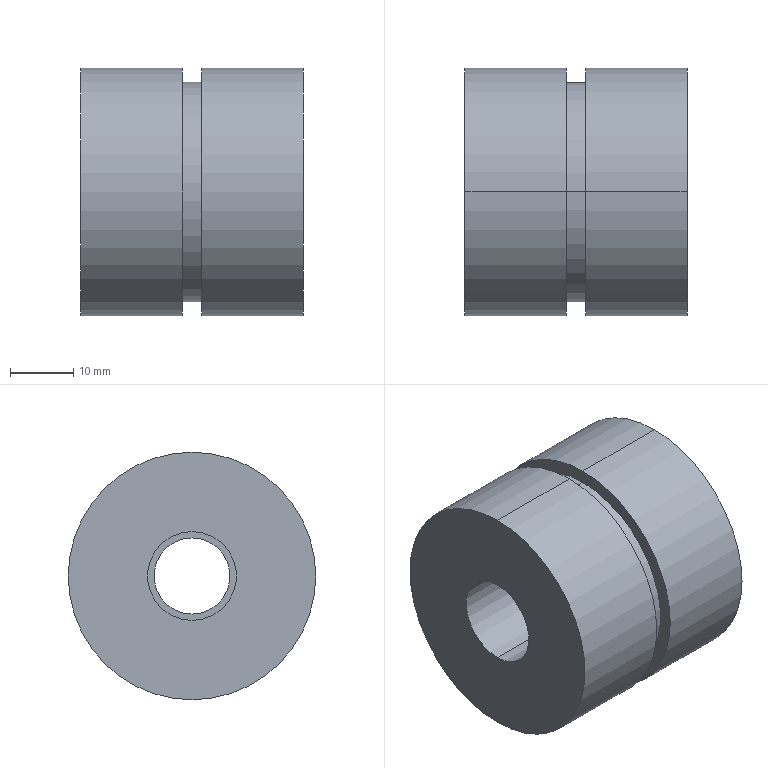Part | STEP file | PN_0042 single diaphragm coupling 39-35-14-12 | 1 solid | 15 faces | box 35 x 39 x 39 mm | volume 36443 mm3 | cylinder 10 | plane 5 | commonest cylinder face diameters 39 x4 12 x2 14 x2 34.646 x2
STEP:
#1=CARTESIAN_POINT('',(0.,0.,0.));
#2=DIRECTION('',(0.,0.,1.));
#3=DIRECTION('',(1.,0.,0.));
#4=AXIS2_PLACEMENT_3D('',#1,#2,#3);
#5=CARTESIAN_POINT('',(1.5,0.,17.323));
#6=VERTEX_POINT('',#5);
#7=CARTESIAN_POINT('',(1.5,0.,-17.323));
#8=VERTEX_POINT('',#7);
#9=CARTESIAN_POINT('',(1.5,0.,0.));
#10=DIRECTION('',(-1.,0.,0.));
#11=DIRECTION('',(0.,0.,1.));
#12=AXIS2_PLACEMENT_3D('',#9,#10,#11);
#13=CIRCLE('',#12,17.323);
#14=CARTESIAN_POINT('',(0.,0.,0.));
#15=DIRECTION('',(-1.,0.,0.));
#16=DIRECTION('',(0.,0.,1.));
#17=AXIS2_PLACEMENT_3D('',#14,#15,#16);
#18=CYLINDRICAL_SURFACE('',#17,17.323);
#19=CARTESIAN_POINT('',(0.,-1.5));
#20=DIRECTION('',(1.,0.));
#21=VECTOR('',#20,1.);
#22=LINE('',#19,#21);
#23=(GEOMETRIC_REPRESENTATION_CONTEXT(2)PARAMETRIC_REPRESENTATION_CONTEXT()REPRESENTATION_CONTEXT('',''));
#24=DEFINITIONAL_REPRESENTATION('',(#22),#23);
#25=PCURVE('',#18,#24);
#26=CARTESIAN_POINT('',(1.5,0.,20.859));
#27=DIRECTION('',(1.,0.,0.));
#28=DIRECTION('',(0.,0.,-1.));
#29=AXIS2_PLACEMENT_3D('',#26,#27,#28);
#30=PLANE('',#29);
#31=CARTESIAN_POINT('',(3.536,0.));
#32=CARTESIAN_POINT('',(3.536,30.004));
#33=CARTESIAN_POINT('',(29.52,15.002));
#34=CARTESIAN_POINT('',(55.505,0.));
#35=CARTESIAN_POINT('',(29.52,-15.002));
#36=CARTESIAN_POINT('',(3.536,-30.004));
#37=CARTESIAN_POINT('',(3.536,0.));
#38=(BOUNDED_CURVE()B_SPLINE_CURVE(2,(#31,#32,#33,#34,#35,#36,#37),.UNSPECIFIED.,.T.,.F.)B_SPLINE_CURVE_WITH_KNOTS((1,2,2,2,2,1),(-2.094,0.,2.094,4.189,6.283,8.378),.UNSPECIFIED.)CURVE()GEOMETRIC_REPRESENTATION_ITEM()RATIONAL_B_SPLINE_CURVE((1.,0.5,1.,0.5,1.,0.5,1.))REPRESENTATION_ITEM(''));
#39=(GEOMETRIC_REPRESENTATION_CONTEXT(2)PARAMETRIC_REPRESENTATION_CONTEXT()REPRESENTATION_CONTEXT('',''));
#40=DEFINITIONAL_REPRESENTATION('',(#38),#39);
#41=PCURVE('',#30,#40);
#42=SURFACE_CURVE('',#13,(#25,#41),.PCURVE_S1.);
#43=EDGE_CURVE('',#6,#8,#42,.T.);
#44=ORIENTED_EDGE('',*,*,#43,.T.);
#45=CARTESIAN_POINT('',(-1.5,0.,-17.323));
#46=VERTEX_POINT('',#45);
#47=CARTESIAN_POINT('',(0.,0.,-17.323));
#48=DIRECTION('',(-1.,0.,0.));
#49=VECTOR('',#48,1.);
#50=LINE('',#47,#49);
#51=CARTESIAN_POINT('',(3.142,0.));
#52=DIRECTION('',(0.,1.));
#53=VECTOR('',#52,1.);
#54=LINE('',#51,#53);
#55=(GEOMETRIC_REPRESENTATION_CONTEXT(2)PARAMETRIC_REPRESENTATION_CONTEXT()REPRESENTATION_CONTEXT('',''));
#56=DEFINITIONAL_REPRESENTATION('',(#54),#55);
#57=PCURVE('',#18,#56);
#58=CARTESIAN_POINT('',(0.,0.,0.));
#59=DIRECTION('',(-1.,0.,0.));
#60=DIRECTION('',(0.,0.,1.));
#61=AXIS2_PLACEMENT_3D('',#58,#59,#60);
#62=CYLINDRICAL_SURFACE('',#61,17.323);
#63=CARTESIAN_POINT('',(3.142,0.));
#64=DIRECTION('',(0.,1.));
#65=VECTOR('',#64,1.);
#66=LINE('',#63,#65);
#67=(GEOMETRIC_REPRESENTATION_CONTEXT(2)PARAMETRIC_REPRESENTATION_CONTEXT()REPRESENTATION_CONTEXT('',''));
#68=DEFINITIONAL_REPRESENTATION('',(#66),#67);
#69=PCURVE('',#62,#68);
#70=SURFACE_CURVE('',#50,(#57,#69),.PCURVE_S1.);
#71=EDGE_CURVE('',#8,#46,#70,.T.);
#72=ORIENTED_EDGE('',*,*,#71,.T.);
#73=CARTESIAN_POINT('',(-1.5,0.,17.323));
#74=VERTEX_POINT('',#73);
#75=CARTESIAN_POINT('',(-1.5,0.,0.));
#76=DIRECTION('',(-1.,0.,0.));
#77=DIRECTION('',(0.,0.,1.));
#78=AXIS2_PLACEMENT_3D('',#75,#76,#77);
#79=CIRCLE('',#78,17.323);
#80=CARTESIAN_POINT('',(0.,1.5));
#81=DIRECTION('',(1.,0.));
#82=VECTOR('',#81,1.);
#83=LINE('',#80,#82);
#84=(GEOMETRIC_REPRESENTATION_CONTEXT(2)PARAMETRIC_REPRESENTATION_CONTEXT()REPRESENTATION_CONTEXT('',''));
#85=DEFINITIONAL_REPRESENTATION('',(#83),#84);
#86=PCURVE('',#18,#85);
#87=CARTESIAN_POINT('',(-1.5,0.,20.859));
#88=DIRECTION('',(-1.,0.,0.));
#89=DIRECTION('',(0.,0.,1.));
#90=AXIS2_PLACEMENT_3D('',#87,#88,#89);
#91=PLANE('',#90);
#92=CARTESIAN_POINT('',(-20.859,0.));
#93=DIRECTION('',(1.,0.));
#94=AXIS2_PLACEMENT_2D('',#92,#93);
#95=CIRCLE('',#94,17.323);
#96=(GEOMETRIC_REPRESENTATION_CONTEXT(2)PARAMETRIC_REPRESENTATION_CONTEXT()REPRESENTATION_CONTEXT('',''));
#97=DEFINITIONAL_REPRESENTATION('',(#95),#96);
#98=PCURVE('',#91,#97);
#99=SURFACE_CURVE('',#79,(#86,#98),.PCURVE_S1.);
#100=EDGE_CURVE('',#74,#46,#99,.T.);
#101=ORIENTED_EDGE('',*,*,#100,.F.);
#102=CARTESIAN_POINT('',(0.,0.,17.323));
#103=DIRECTION('',(-1.,0.,0.));
#104=VECTOR('',#103,1.);
#105=LINE('',#102,#104);
#106=CARTESIAN_POINT('',(0.,0.));
#107=DIRECTION('',(0.,1.));
#108=VECTOR('',#107,1.);
#109=LINE('',#106,#108);
#110=(GEOMETRIC_REPRESENTATION_CONTEXT(2)PARAMETRIC_REPRESENTATION_CONTEXT()REPRESENTATION_CONTEXT('',''));
#111=DEFINITIONAL_REPRESENTATION('',(#109),#110);
#112=PCURVE('',#18,#111);
#113=CARTESIAN_POINT('',(6.283,0.));
#114=DIRECTION('',(0.,1.));
#115=VECTOR('',#114,1.);
#116=LINE('',#113,#115);
#117=(GEOMETRIC_REPRESENTATION_CONTEXT(2)PARAMETRIC_REPRESENTATION_CONTEXT()REPRESENTATION_CONTEXT('',''));
#118=DEFINITIONAL_REPRESENTATION('',(#116),#117);
#119=PCURVE('',#62,#118);
#120=SURFACE_CURVE('',#105,(#112,#119),.PCURVE_S1.);
#121=EDGE_CURVE('',#6,#74,#120,.T.);
#122=ORIENTED_EDGE('',*,*,#121,.F.);
#123=EDGE_LOOP('',(#44,#72,#101,#122));
#124=FACE_BOUND('',#123,.T.);
#125=ADVANCED_FACE('',(#124),#18,.T.);
#126=CARTESIAN_POINT('',(-1.5,0.,7.));
#127=VERTEX_POINT('',#126);
#128=CARTESIAN_POINT('',(-17.5,0.,7.));
#129=VERTEX_POINT('',#128);
#130=CARTESIAN_POINT('',(-1.5,0.,7.));
#131=DIRECTION('',(-1.,0.,0.));
#132=VECTOR('',#131,1.);
#133=LINE('',#130,#132);
#134=CARTESIAN_POINT('',(-1.5,0.,0.));
#135=DIRECTION('',(-1.,0.,0.));
#136=DIRECTION('',(0.,0.,1.));
#137=AXIS2_PLACEMENT_3D('',#134,#135,#136);
#138=CYLINDRICAL_SURFACE('',#137,7.);
#139=CARTESIAN_POINT('',(6.283,0.));
#140=DIRECTION('',(0.,1.));
#141=VECTOR('',#140,1.);
#142=LINE('',#139,#141);
#143=(GEOMETRIC_REPRESENTATION_CONTEXT(2)PARAMETRIC_REPRESENTATION_CONTEXT()REPRESENTATION_CONTEXT('',''));
#144=DEFINITIONAL_REPRESENTATION('',(#142),#143);
#145=PCURVE('',#138,#144);
#146=CARTESIAN_POINT('',(-1.5,0.,0.));
#147=DIRECTION('',(-1.,0.,0.));
#148=DIRECTION('',(0.,0.,1.));
#149=AXIS2_PLACEMENT_3D('',#146,#147,#148);
#150=CYLINDRICAL_SURFACE('',#149,7.);
#151=CARTESIAN_POINT('',(0.,0.));
#152=DIRECTION('',(0.,1.));
#153=VECTOR('',#152,1.);
#154=LINE('',#151,#153);
#155=(GEOMETRIC_REPRESENTATION_CONTEXT(2)PARAMETRIC_REPRESENTATION_CONTEXT()REPRESENTATION_CONTEXT('',''));
#156=DEFINITIONAL_REPRESENTATION('',(#154),#155);
#157=PCURVE('',#150,#156);
#158=SURFACE_CURVE('',#133,(#145,#157),.PCURVE_S1.);
#159=EDGE_CURVE('',#127,#129,#158,.T.);
#160=ORIENTED_EDGE('',*,*,#159,.T.);
#161=CARTESIAN_POINT('',(-17.5,0.,-7.));
#162=VERTEX_POINT('',#161);
#163=CARTESIAN_POINT('',(-17.5,0.,0.));
#164=DIRECTION('',(-1.,0.,0.));
#165=DIRECTION('',(0.,0.,1.));
#166=AXIS2_PLACEMENT_3D('',#163,#164,#165);
#167=CIRCLE('',#166,7.);
#168=CARTESIAN_POINT('',(0.,16.));
#169=DIRECTION('',(1.,0.));
#170=VECTOR('',#169,1.);
#171=LINE('',#168,#170);
#172=(GEOMETRIC_REPRESENTATION_CONTEXT(2)PARAMETRIC_REPRESENTATION_CONTEXT()REPRESENTATION_CONTEXT('',''));
#173=DEFINITIONAL_REPRESENTATION('',(#171),#172);
#174=PCURVE('',#138,#173);
#175=CARTESIAN_POINT('',(-17.5,0.,0.));
#176=DIRECTION('',(1.,0.,0.));
#177=DIRECTION('',(0.,0.,-1.));
#178=AXIS2_PLACEMENT_3D('',#175,#176,#177);
#179=PLANE('',#178);
#180=CARTESIAN_POINT('',(-7.,0.));
#181=CARTESIAN_POINT('',(-7.,12.124));
#182=CARTESIAN_POINT('',(3.5,6.062));
#183=CARTESIAN_POINT('',(14.,0.));
#184=CARTESIAN_POINT('',(3.5,-6.062));
#185=CARTESIAN_POINT('',(-7.,-12.124));
#186=CARTESIAN_POINT('',(-7.,0.));
#187=(BOUNDED_CURVE()B_SPLINE_CURVE(2,(#180,#181,#182,#183,#184,#185,#186),.UNSPECIFIED.,.T.,.F.)B_SPLINE_CURVE_WITH_KNOTS((1,2,2,2,2,1),(-2.094,0.,2.094,4.189,6.283,8.378),.UNSPECIFIED.)CURVE()GEOMETRIC_REPRESENTATION_ITEM()RATIONAL_B_SPLINE_CURVE((1.,0.5,1.,0.5,1.,0.5,1.))REPRESENTATION_ITEM(''));
#188=(GEOMETRIC_REPRESENTATION_CONTEXT(2)PARAMETRIC_REPRESENTATION_CONTEXT()REPRESENTATION_CONTEXT('',''));
#189=DEFINITIONAL_REPRESENTATION('',(#187),#188);
#190=PCURVE('',#179,#189);
#191=SURFACE_CURVE('',#167,(#174,#190),.PCURVE_S1.);
#192=EDGE_CURVE('',#162,#129,#191,.T.);
#193=ORIENTED_EDGE('',*,*,#192,.F.);
#194=CARTESIAN_POINT('',(-1.5,0.,-7.));
#195=VERTEX_POINT('',#194);
#196=CARTESIAN_POINT('',(-1.5,0.,-7.));
#197=DIRECTION('',(-1.,0.,0.));
#198=VECTOR('',#197,1.);
#199=LINE('',#196,#198);
#200=CARTESIAN_POINT('',(3.142,0.));
#201=DIRECTION('',(0.,1.));
#202=VECTOR('',#201,1.);
#203=LINE('',#200,#202);
#204=(GEOMETRIC_REPRESENTATION_CONTEXT(2)PARAMETRIC_REPRESENTATION_CONTEXT()REPRESENTATION_CONTEXT('',''));
#205=DEFINITIONAL_REPRESENTATION('',(#203),#204);
#206=PCURVE('',#138,#205);
#207=CARTESIAN_POINT('',(3.142,0.));
#208=DIRECTION('',(0.,1.));
#209=VECTOR('',#208,1.);
#210=LINE('',#207,#209);
#211=(GEOMETRIC_REPRESENTATION_CONTEXT(2)PARAMETRIC_REPRESENTATION_CONTEXT()REPRESENTATION_CONTEXT('',''));
#212=DEFINITIONAL_REPRESENTATION('',(#210),#211);
#213=PCURVE('',#150,#212);
#214=SURFACE_CURVE('',#199,(#206,#213),.PCURVE_S1.);
#215=EDGE_CURVE('',#195,#162,#214,.T.);
#216=ORIENTED_EDGE('',*,*,#215,.F.);
#217=CARTESIAN_POINT('',(-1.5,0.,0.));
#218=DIRECTION('',(-1.,0.,0.));
#219=DIRECTION('',(0.,0.,1.));
#220=AXIS2_PLACEMENT_3D('',#217,#218,#219);
#221=CIRCLE('',#220,7.);
#222=CARTESIAN_POINT('',(0.,0.));
#223=DIRECTION('',(1.,0.));
#224=VECTOR('',#223,1.);
#225=LINE('',#222,#224);
#226=(GEOMETRIC_REPRESENTATION_CONTEXT(2)PARAMETRIC_REPRESENTATION_CONTEXT()REPRESENTATION_CONTEXT('',''));
#227=DEFINITIONAL_REPRESENTATION('',(#225),#226);
#228=PCURVE('',#138,#227);
#229=CARTESIAN_POINT('',(-1.5,0.,0.));
#230=DIRECTION('',(-1.,0.,0.));
#231=DIRECTION('',(0.,0.,1.));
#232=AXIS2_PLACEMENT_3D('',#229,#230,#231);
#233=PLANE('',#232);
#234=CARTESIAN_POINT('',(0.,0.));
#235=DIRECTION('',(1.,0.));
#236=AXIS2_PLACEMENT_2D('',#234,#235);
#237=CIRCLE('',#236,7.);
#238=(GEOMETRIC_REPRESENTATION_CONTEXT(2)PARAMETRIC_REPRESENTATION_CONTEXT()REPRESENTATION_CONTEXT('',''));
#239=DEFINITIONAL_REPRESENTATION('',(#237),#238);
#240=PCURVE('',#233,#239);
#241=SURFACE_CURVE('',#221,(#228,#240),.PCURVE_S1.);
#242=EDGE_CURVE('',#195,#127,#241,.T.);
#243=ORIENTED_EDGE('',*,*,#242,.T.);
#244=EDGE_LOOP('',(#160,#193,#216,#243));
#245=FACE_BOUND('',#244,.F.);
#246=ADVANCED_FACE('',(#245),#138,.F.);
#247=CARTESIAN_POINT('',(17.5,0.,-19.5));
#248=VERTEX_POINT('',#247);
#249=CARTESIAN_POINT('',(17.5,0.,19.5));
#250=VERTEX_POINT('',#249);
#251=CARTESIAN_POINT('',(17.5,0.,0.));
#252=DIRECTION('',(1.,0.,0.));
#253=DIRECTION('',(0.,0.,-1.));
#254=AXIS2_PLACEMENT_3D('',#251,#252,#253);
#255=CIRCLE('',#254,19.5);
#256=CARTESIAN_POINT('',(17.5,0.,0.));
#257=DIRECTION('',(-1.,0.,0.));
#258=DIRECTION('',(0.,0.,1.));
#259=AXIS2_PLACEMENT_3D('',#256,#257,#258);
#260=CYLINDRICAL_SURFACE('',#259,19.5);
#261=CARTESIAN_POINT('',(3.142,0.));
#262=DIRECTION('',(-1.,0.));
#263=VECTOR('',#262,1.);
#264=LINE('',#261,#263);
#265=(GEOMETRIC_REPRESENTATION_CONTEXT(2)PARAMETRIC_REPRESENTATION_CONTEXT()REPRESENTATION_CONTEXT('',''));
#266=DEFINITIONAL_REPRESENTATION('',(#264),#265);
#267=PCURVE('',#260,#266);
#268=CARTESIAN_POINT('',(17.5,0.,0.));
#269=DIRECTION('',(1.,0.,0.));
#270=DIRECTION('',(0.,0.,-1.));
#271=AXIS2_PLACEMENT_3D('',#268,#269,#270);
#272=PLANE('',#271);
#273=CARTESIAN_POINT('',(0.,0.));
#274=DIRECTION('',(1.,0.));
#275=AXIS2_PLACEMENT_2D('',#273,#274);
#276=CIRCLE('',#275,19.5);
#277=(GEOMETRIC_REPRESENTATION_CONTEXT(2)PARAMETRIC_REPRESENTATION_CONTEXT()REPRESENTATION_CONTEXT('',''));
#278=DEFINITIONAL_REPRESENTATION('',(#276),#277);
#279=PCURVE('',#272,#278);
#280=SURFACE_CURVE('',#255,(#267,#279),.PCURVE_S1.);
#281=EDGE_CURVE('',#248,#250,#280,.T.);
#282=ORIENTED_EDGE('',*,*,#281,.F.);
#283=CARTESIAN_POINT('',(1.5,0.,-19.5));
#284=VERTEX_POINT('',#283);
#285=CARTESIAN_POINT('',(17.5,0.,-19.5));
#286=DIRECTION('',(-1.,0.,0.));
#287=VECTOR('',#286,1.);
#288=LINE('',#285,#287);
#289=CARTESIAN_POINT('',(3.142,0.));
#290=DIRECTION('',(0.,1.));
#291=VECTOR('',#290,1.);
#292=LINE('',#289,#291);
#293=(GEOMETRIC_REPRESENTATION_CONTEXT(2)PARAMETRIC_REPRESENTATION_CONTEXT()REPRESENTATION_CONTEXT('',''));
#294=DEFINITIONAL_REPRESENTATION('',(#292),#293);
#295=PCURVE('',#260,#294);
#296=CARTESIAN_POINT('',(17.5,0.,0.));
#297=DIRECTION('',(-1.,0.,0.));
#298=DIRECTION('',(0.,0.,1.));
#299=AXIS2_PLACEMENT_3D('',#296,#297,#298);
#300=CYLINDRICAL_SURFACE('',#299,19.5);
#301=CARTESIAN_POINT('',(3.142,0.));
#302=DIRECTION('',(0.,1.));
#303=VECTOR('',#302,1.);
#304=LINE('',#301,#303);
#305=(GEOMETRIC_REPRESENTATION_CONTEXT(2)PARAMETRIC_REPRESENTATION_CONTEXT()REPRESENTATION_CONTEXT('',''));
#306=DEFINITIONAL_REPRESENTATION('',(#304),#305);
#307=PCURVE('',#300,#306);
#308=SURFACE_CURVE('',#288,(#295,#307),.PCURVE_S1.);
#309=EDGE_CURVE('',#248,#284,#308,.T.);
#310=ORIENTED_EDGE('',*,*,#309,.T.);
#311=CARTESIAN_POINT('',(1.5,0.,19.5));
#312=VERTEX_POINT('',#311);
#313=CARTESIAN_POINT('',(1.5,0.,0.));
#314=DIRECTION('',(1.,0.,0.));
#315=DIRECTION('',(0.,0.,-1.));
#316=AXIS2_PLACEMENT_3D('',#313,#314,#315);
#317=CIRCLE('',#316,19.5);
#318=CARTESIAN_POINT('',(3.142,16.));
#319=DIRECTION('',(-1.,0.));
#320=VECTOR('',#319,1.);
#321=LINE('',#318,#320);
#322=(GEOMETRIC_REPRESENTATION_CONTEXT(2)PARAMETRIC_REPRESENTATION_CONTEXT()REPRESENTATION_CONTEXT('',''));
#323=DEFINITIONAL_REPRESENTATION('',(#321),#322);
#324=PCURVE('',#260,#323);
#325=CARTESIAN_POINT('',(20.859,0.));
#326=DIRECTION('',(1.,0.));
#327=AXIS2_PLACEMENT_2D('',#325,#326);
#328=CIRCLE('',#327,19.5);
#329=(GEOMETRIC_REPRESENTATION_CONTEXT(2)PARAMETRIC_REPRESENTATION_CONTEXT()REPRESENTATION_CONTEXT('',''));
#330=DEFINITIONAL_REPRESENTATION('',(#328),#329);
#331=PCURVE('',#30,#330);
#332=SURFACE_CURVE('',#317,(#324,#331),.PCURVE_S1.);
#333=EDGE_CURVE('',#284,#312,#332,.T.);
#334=ORIENTED_EDGE('',*,*,#333,.T.);
#335=CARTESIAN_POINT('',(17.5,0.,19.5));
#336=DIRECTION('',(-1.,0.,0.));
#337=VECTOR('',#336,1.);
#338=LINE('',#335,#337);
#339=CARTESIAN_POINT('',(0.,0.));
#340=DIRECTION('',(0.,1.));
#341=VECTOR('',#340,1.);
#342=LINE('',#339,#341);
#343=(GEOMETRIC_REPRESENTATION_CONTEXT(2)PARAMETRIC_REPRESENTATION_CONTEXT()REPRESENTATION_CONTEXT('',''));
#344=DEFINITIONAL_REPRESENTATION('',(#342),#343);
#345=PCURVE('',#260,#344);
#346=CARTESIAN_POINT('',(6.283,0.));
#347=DIRECTION('',(0.,1.));
#348=VECTOR('',#347,1.);
#349=LINE('',#346,#348);
#350=(GEOMETRIC_REPRESENTATION_CONTEXT(2)PARAMETRIC_REPRESENTATION_CONTEXT()REPRESENTATION_CONTEXT('',''));
#351=DEFINITIONAL_REPRESENTATION('',(#349),#350);
#352=PCURVE('',#300,#351);
#353=SURFACE_CURVE('',#338,(#345,#352),.PCURVE_S1.);
#354=EDGE_CURVE('',#250,#312,#353,.T.);
#355=ORIENTED_EDGE('',*,*,#354,.F.);
#356=EDGE_LOOP('',(#282,#310,#334,#355));
#357=FACE_BOUND('',#356,.T.);
#358=ADVANCED_FACE('',(#357),#260,.T.);
#359=CARTESIAN_POINT('',(-1.5,0.,-6.));
#360=VERTEX_POINT('',#359);
#361=CARTESIAN_POINT('',(17.5,0.,-6.));
#362=VERTEX_POINT('',#361);
#363=CARTESIAN_POINT('',(-17.5,0.,-6.));
#364=DIRECTION('',(1.,0.,0.));
#365=VECTOR('',#364,1.);
#366=LINE('',#363,#365);
#367=CARTESIAN_POINT('',(-17.5,0.,0.));
#368=DIRECTION('',(1.,0.,0.));
#369=DIRECTION('',(0.,0.,-1.));
#370=AXIS2_PLACEMENT_3D('',#367,#368,#369);
#371=CYLINDRICAL_SURFACE('',#370,6.);
#372=CARTESIAN_POINT('',(6.283,0.));
#373=DIRECTION('',(0.,1.));
#374=VECTOR('',#373,1.);
#375=LINE('',#372,#374);
#376=(GEOMETRIC_REPRESENTATION_CONTEXT(2)PARAMETRIC_REPRESENTATION_CONTEXT()REPRESENTATION_CONTEXT('',''));
#377=DEFINITIONAL_REPRESENTATION('',(#375),#376);
#378=PCURVE('',#371,#377);
#379=CARTESIAN_POINT('',(-17.5,0.,0.));
#380=DIRECTION('',(1.,0.,0.));
#381=DIRECTION('',(0.,0.,-1.));
#382=AXIS2_PLACEMENT_3D('',#379,#380,#381);
#383=CYLINDRICAL_SURFACE('',#382,6.);
#384=CARTESIAN_POINT('',(0.,0.));
#385=DIRECTION('',(0.,1.));
#386=VECTOR('',#385,1.);
#387=LINE('',#384,#386);
#388=(GEOMETRIC_REPRESENTATION_CONTEXT(2)PARAMETRIC_REPRESENTATION_CONTEXT()REPRESENTATION_CONTEXT('',''));
#389=DEFINITIONAL_REPRESENTATION('',(#387),#388);
#390=PCURVE('',#383,#389);
#391=SURFACE_CURVE('',#366,(#378,#390),.PCURVE_S1.);
#392=EDGE_CURVE('',#360,#362,#391,.T.);
#393=ORIENTED_EDGE('',*,*,#392,.T.);
#394=CARTESIAN_POINT('',(17.5,0.,6.));
#395=VERTEX_POINT('',#394);
#396=CARTESIAN_POINT('',(17.5,0.,0.));
#397=DIRECTION('',(1.,0.,0.));
#398=DIRECTION('',(0.,0.,-1.));
#399=AXIS2_PLACEMENT_3D('',#396,#397,#398);
#400=CIRCLE('',#399,6.);
#401=CARTESIAN_POINT('',(0.,35.));
#402=DIRECTION('',(1.,0.));
#403=VECTOR('',#402,1.);
#404=LINE('',#401,#403);
#405=(GEOMETRIC_REPRESENTATION_CONTEXT(2)PARAMETRIC_REPRESENTATION_CONTEXT()REPRESENTATION_CONTEXT('',''));
#406=DEFINITIONAL_REPRESENTATION('',(#404),#405);
#407=PCURVE('',#371,#406);
#408=CARTESIAN_POINT('',(0.,0.));
#409=DIRECTION('',(1.,0.));
#410=AXIS2_PLACEMENT_2D('',#408,#409);
#411=CIRCLE('',#410,6.);
#412=(GEOMETRIC_REPRESENTATION_CONTEXT(2)PARAMETRIC_REPRESENTATION_CONTEXT()REPRESENTATION_CONTEXT('',''));
#413=DEFINITIONAL_REPRESENTATION('',(#411),#412);
#414=PCURVE('',#272,#413);
#415=SURFACE_CURVE('',#400,(#407,#414),.PCURVE_S1.);
#416=EDGE_CURVE('',#395,#362,#415,.T.);
#417=ORIENTED_EDGE('',*,*,#416,.F.);
#418=CARTESIAN_POINT('',(-1.5,0.,6.));
#419=VERTEX_POINT('',#418);
#420=CARTESIAN_POINT('',(-17.5,0.,6.));
#421=DIRECTION('',(1.,0.,0.));
#422=VECTOR('',#421,1.);
#423=LINE('',#420,#422);
#424=CARTESIAN_POINT('',(3.142,0.));
#425=DIRECTION('',(0.,1.));
#426=VECTOR('',#425,1.);
#427=LINE('',#424,#426);
#428=(GEOMETRIC_REPRESENTATION_CONTEXT(2)PARAMETRIC_REPRESENTATION_CONTEXT()REPRESENTATION_CONTEXT('',''));
#429=DEFINITIONAL_REPRESENTATION('',(#427),#428);
#430=PCURVE('',#371,#429);
#431=CARTESIAN_POINT('',(3.142,0.));
#432=DIRECTION('',(0.,1.));
#433=VECTOR('',#432,1.);
#434=LINE('',#431,#433);
#435=(GEOMETRIC_REPRESENTATION_CONTEXT(2)PARAMETRIC_REPRESENTATION_CONTEXT()REPRESENTATION_CONTEXT('',''));
#436=DEFINITIONAL_REPRESENTATION('',(#434),#435);
#437=PCURVE('',#383,#436);
#438=SURFACE_CURVE('',#423,(#430,#437),.PCURVE_S1.);
#439=EDGE_CURVE('',#419,#395,#438,.T.);
#440=ORIENTED_EDGE('',*,*,#439,.F.);
#441=CARTESIAN_POINT('',(-1.5,0.,0.));
#442=DIRECTION('',(1.,0.,0.));
#443=DIRECTION('',(0.,0.,1.));
#444=AXIS2_PLACEMENT_3D('',#441,#442,#443);
#445=CIRCLE('',#444,6.);
#446=CARTESIAN_POINT('',(3.142,16.));
#447=DIRECTION('',(1.,0.));
#448=VECTOR('',#447,1.);
#449=LINE('',#446,#448);
#450=(GEOMETRIC_REPRESENTATION_CONTEXT(2)PARAMETRIC_REPRESENTATION_CONTEXT()REPRESENTATION_CONTEXT('',''));
#451=DEFINITIONAL_REPRESENTATION('',(#449),#450);
#452=PCURVE('',#371,#451);
#453=CARTESIAN_POINT('',(6.,0.));
#454=CARTESIAN_POINT('',(6.,-10.392));
#455=CARTESIAN_POINT('',(-3.,-5.196));
#456=CARTESIAN_POINT('',(-12.,0.));
#457=CARTESIAN_POINT('',(-3.,5.196));
#458=CARTESIAN_POINT('',(6.,10.392));
#459=CARTESIAN_POINT('',(6.,0.));
#460=(BOUNDED_CURVE()B_SPLINE_CURVE(2,(#453,#454,#455,#456,#457,#458,#459),.UNSPECIFIED.,.T.,.F.)B_SPLINE_CURVE_WITH_KNOTS((1,2,2,2,2,1),(-2.094,0.,2.094,4.189,6.283,8.378),.UNSPECIFIED.)CURVE()GEOMETRIC_REPRESENTATION_ITEM()RATIONAL_B_SPLINE_CURVE((1.,0.5,1.,0.5,1.,0.5,1.))REPRESENTATION_ITEM(''));
#461=(GEOMETRIC_REPRESENTATION_CONTEXT(2)PARAMETRIC_REPRESENTATION_CONTEXT()REPRESENTATION_CONTEXT('',''));
#462=DEFINITIONAL_REPRESENTATION('',(#460),#461);
#463=PCURVE('',#233,#462);
#464=SURFACE_CURVE('',#445,(#452,#463),.PCURVE_S1.);
#465=EDGE_CURVE('',#419,#360,#464,.T.);
#466=ORIENTED_EDGE('',*,*,#465,.T.);
#467=EDGE_LOOP('',(#393,#417,#440,#466));
#468=FACE_BOUND('',#467,.F.);
#469=ADVANCED_FACE('',(#468),#371,.F.);
#470=CARTESIAN_POINT('',(-1.5,0.,19.5));
#471=VERTEX_POINT('',#470);
#472=CARTESIAN_POINT('',(-1.5,0.,-19.5));
#473=VERTEX_POINT('',#472);
#474=CARTESIAN_POINT('',(-1.5,0.,0.));
#475=DIRECTION('',(-1.,0.,0.));
#476=DIRECTION('',(0.,0.,1.));
#477=AXIS2_PLACEMENT_3D('',#474,#475,#476);
#478=CIRCLE('',#477,19.5);
#479=CARTESIAN_POINT('',(17.5,0.,0.));
#480=DIRECTION('',(-1.,0.,0.));
#481=DIRECTION('',(0.,0.,1.));
#482=AXIS2_PLACEMENT_3D('',#479,#480,#481);
#483=CYLINDRICAL_SURFACE('',#482,19.5);
#484=CARTESIAN_POINT('',(0.,19.));
#485=DIRECTION('',(1.,0.));
#486=VECTOR('',#485,1.);
#487=LINE('',#484,#486);
#488=(GEOMETRIC_REPRESENTATION_CONTEXT(2)PARAMETRIC_REPRESENTATION_CONTEXT()REPRESENTATION_CONTEXT('',''));
#489=DEFINITIONAL_REPRESENTATION('',(#487),#488);
#490=PCURVE('',#483,#489);
#491=CARTESIAN_POINT('',(-20.859,0.));
#492=DIRECTION('',(1.,0.));
#493=AXIS2_PLACEMENT_2D('',#491,#492);
#494=CIRCLE('',#493,19.5);
#495=(GEOMETRIC_REPRESENTATION_CONTEXT(2)PARAMETRIC_REPRESENTATION_CONTEXT()REPRESENTATION_CONTEXT('',''));
#496=DEFINITIONAL_REPRESENTATION('',(#494),#495);
#497=PCURVE('',#91,#496);
#498=SURFACE_CURVE('',#478,(#490,#497),.PCURVE_S1.);
#499=EDGE_CURVE('',#471,#473,#498,.T.);
#500=ORIENTED_EDGE('',*,*,#499,.T.);
#501=CARTESIAN_POINT('',(-17.5,0.,-19.5));
#502=VERTEX_POINT('',#501);
#503=CARTESIAN_POINT('',(17.5,0.,-19.5));
#504=DIRECTION('',(-1.,0.,0.));
#505=VECTOR('',#504,1.);
#506=LINE('',#503,#505);
#507=CARTESIAN_POINT('',(3.142,0.));
#508=DIRECTION('',(0.,1.));
#509=VECTOR('',#508,1.);
#510=LINE('',#507,#509);
#511=(GEOMETRIC_REPRESENTATION_CONTEXT(2)PARAMETRIC_REPRESENTATION_CONTEXT()REPRESENTATION_CONTEXT('',''));
#512=DEFINITIONAL_REPRESENTATION('',(#510),#511);
#513=PCURVE('',#483,#512);
#514=CARTESIAN_POINT('',(17.5,0.,0.));
#515=DIRECTION('',(-1.,0.,0.));
#516=DIRECTION('',(0.,0.,1.));
#517=AXIS2_PLACEMENT_3D('',#514,#515,#516);
#518=CYLINDRICAL_SURFACE('',#517,19.5);
#519=CARTESIAN_POINT('',(3.142,0.));
#520=DIRECTION('',(0.,1.));
#521=VECTOR('',#520,1.);
#522=LINE('',#519,#521);
#523=(GEOMETRIC_REPRESENTATION_CONTEXT(2)PARAMETRIC_REPRESENTATION_CONTEXT()REPRESENTATION_CONTEXT('',''));
#524=DEFINITIONAL_REPRESENTATION('',(#522),#523);
#525=PCURVE('',#518,#524);
#526=SURFACE_CURVE('',#506,(#513,#525),.PCURVE_S1.);
#527=EDGE_CURVE('',#473,#502,#526,.T.);
#528=ORIENTED_EDGE('',*,*,#527,.T.);
#529=CARTESIAN_POINT('',(-17.5,0.,19.5));
#530=VERTEX_POINT('',#529);
#531=CARTESIAN_POINT('',(-17.5,0.,0.));
#532=DIRECTION('',(1.,0.,0.));
#533=DIRECTION('',(0.,0.,-1.));
#534=AXIS2_PLACEMENT_3D('',#531,#532,#533);
#535=CIRCLE('',#534,19.5);
#536=CARTESIAN_POINT('',(3.142,35.));
#537=DIRECTION('',(-1.,0.));
#538=VECTOR('',#537,1.);
#539=LINE('',#536,#538);
#540=(GEOMETRIC_REPRESENTATION_CONTEXT(2)PARAMETRIC_REPRESENTATION_CONTEXT()REPRESENTATION_CONTEXT('',''));
#541=DEFINITIONAL_REPRESENTATION('',(#539),#540);
#542=PCURVE('',#483,#541);
#543=CARTESIAN_POINT('',(0.,0.));
#544=DIRECTION('',(1.,0.));
#545=AXIS2_PLACEMENT_2D('',#543,#544);
#546=CIRCLE('',#545,19.5);
#547=(GEOMETRIC_REPRESENTATION_CONTEXT(2)PARAMETRIC_REPRESENTATION_CONTEXT()REPRESENTATION_CONTEXT('',''));
#548=DEFINITIONAL_REPRESENTATION('',(#546),#547);
#549=PCURVE('',#179,#548);
#550=SURFACE_CURVE('',#535,(#542,#549),.PCURVE_S1.);
#551=EDGE_CURVE('',#502,#530,#550,.T.);
#552=ORIENTED_EDGE('',*,*,#551,.T.);
#553=CARTESIAN_POINT('',(17.5,0.,19.5));
#554=DIRECTION('',(-1.,0.,0.));
#555=VECTOR('',#554,1.);
#556=LINE('',#553,#555);
#557=CARTESIAN_POINT('',(0.,0.));
#558=DIRECTION('',(0.,1.));
#559=VECTOR('',#558,1.);
#560=LINE('',#557,#559);
#561=(GEOMETRIC_REPRESENTATION_CONTEXT(2)PARAMETRIC_REPRESENTATION_CONTEXT()REPRESENTATION_CONTEXT('',''));
#562=DEFINITIONAL_REPRESENTATION('',(#560),#561);
#563=PCURVE('',#483,#562);
#564=CARTESIAN_POINT('',(6.283,0.));
#565=DIRECTION('',(0.,1.));
#566=VECTOR('',#565,1.);
#567=LINE('',#564,#566);
#568=(GEOMETRIC_REPRESENTATION_CONTEXT(2)PARAMETRIC_REPRESENTATION_CONTEXT()REPRESENTATION_CONTEXT('',''));
#569=DEFINITIONAL_REPRESENTATION('',(#567),#568);
#570=PCURVE('',#518,#569);
#571=SURFACE_CURVE('',#556,(#563,#570),.PCURVE_S1.);
#572=EDGE_CURVE('',#471,#530,#571,.T.);
#573=ORIENTED_EDGE('',*,*,#572,.F.);
#574=EDGE_LOOP('',(#500,#528,#552,#573));
#575=FACE_BOUND('',#574,.T.);
#576=ADVANCED_FACE('',(#575),#483,.T.);
#577=ORIENTED_EDGE('',*,*,#527,.F.);
#578=CARTESIAN_POINT('',(-1.5,0.,0.));
#579=DIRECTION('',(-1.,0.,0.));
#580=DIRECTION('',(0.,0.,1.));
#581=AXIS2_PLACEMENT_3D('',#578,#579,#580);
#582=CIRCLE('',#581,19.5);
#583=CARTESIAN_POINT('',(0.,19.));
#584=DIRECTION('',(1.,0.));
#585=VECTOR('',#584,1.);
#586=LINE('',#583,#585);
#587=(GEOMETRIC_REPRESENTATION_CONTEXT(2)PARAMETRIC_REPRESENTATION_CONTEXT()REPRESENTATION_CONTEXT('',''));
#588=DEFINITIONAL_REPRESENTATION('',(#586),#587);
#589=PCURVE('',#518,#588);
#590=CARTESIAN_POINT('',(-20.859,0.));
#591=DIRECTION('',(1.,0.));
#592=AXIS2_PLACEMENT_2D('',#590,#591);
#593=CIRCLE('',#592,19.5);
#594=(GEOMETRIC_REPRESENTATION_CONTEXT(2)PARAMETRIC_REPRESENTATION_CONTEXT()REPRESENTATION_CONTEXT('',''));
#595=DEFINITIONAL_REPRESENTATION('',(#593),#594);
#596=PCURVE('',#91,#595);
#597=SURFACE_CURVE('',#582,(#589,#596),.PCURVE_S1.);
#598=EDGE_CURVE('',#473,#471,#597,.T.);
#599=ORIENTED_EDGE('',*,*,#598,.T.);
#600=ORIENTED_EDGE('',*,*,#572,.T.);
#601=CARTESIAN_POINT('',(-17.5,0.,0.));
#602=DIRECTION('',(1.,0.,0.));
#603=DIRECTION('',(0.,0.,-1.));
#604=AXIS2_PLACEMENT_3D('',#601,#602,#603);
#605=CIRCLE('',#604,19.5);
#606=CARTESIAN_POINT('',(9.425,35.));
#607=DIRECTION('',(-1.,0.));
#608=VECTOR('',#607,1.);
#609=LINE('',#606,#608);
#610=(GEOMETRIC_REPRESENTATION_CONTEXT(2)PARAMETRIC_REPRESENTATION_CONTEXT()REPRESENTATION_CONTEXT('',''));
#611=DEFINITIONAL_REPRESENTATION('',(#609),#610);
#612=PCURVE('',#518,#611);
#613=CARTESIAN_POINT('',(0.,0.));
#614=DIRECTION('',(1.,0.));
#615=AXIS2_PLACEMENT_2D('',#613,#614);
#616=CIRCLE('',#615,19.5);
#617=(GEOMETRIC_REPRESENTATION_CONTEXT(2)PARAMETRIC_REPRESENTATION_CONTEXT()REPRESENTATION_CONTEXT('',''));
#618=DEFINITIONAL_REPRESENTATION('',(#616),#617);
#619=PCURVE('',#179,#618);
#620=SURFACE_CURVE('',#605,(#612,#619),.PCURVE_S1.);
#621=EDGE_CURVE('',#530,#502,#620,.T.);
#622=ORIENTED_EDGE('',*,*,#621,.T.);
#623=EDGE_LOOP('',(#577,#599,#600,#622));
#624=FACE_BOUND('',#623,.T.);
#625=ADVANCED_FACE('',(#624),#518,.T.);
#626=CARTESIAN_POINT('',(17.5,0.,0.));
#627=DIRECTION('',(1.,0.,0.));
#628=DIRECTION('',(0.,0.,-1.));
#629=AXIS2_PLACEMENT_3D('',#626,#627,#628);
#630=CIRCLE('',#629,6.);
#631=CARTESIAN_POINT('',(0.,35.));
#632=DIRECTION('',(1.,0.));
#633=VECTOR('',#632,1.);
#634=LINE('',#631,#633);
#635=(GEOMETRIC_REPRESENTATION_CONTEXT(2)PARAMETRIC_REPRESENTATION_CONTEXT()REPRESENTATION_CONTEXT('',''));
#636=DEFINITIONAL_REPRESENTATION('',(#634),#635);
#637=PCURVE('',#383,#636);
#638=CARTESIAN_POINT('',(0.,0.));
#639=DIRECTION('',(1.,0.));
#640=AXIS2_PLACEMENT_2D('',#638,#639);
#641=CIRCLE('',#640,6.);
#642=(GEOMETRIC_REPRESENTATION_CONTEXT(2)PARAMETRIC_REPRESENTATION_CONTEXT()REPRESENTATION_CONTEXT('',''));
#643=DEFINITIONAL_REPRESENTATION('',(#641),#642);
#644=PCURVE('',#272,#643);
#645=SURFACE_CURVE('',#630,(#637,#644),.PCURVE_S1.);
#646=EDGE_CURVE('',#362,#395,#645,.T.);
#647=ORIENTED_EDGE('',*,*,#646,.F.);
#648=ORIENTED_EDGE('',*,*,#392,.F.);
#649=CARTESIAN_POINT('',(-1.5,0.,0.));
#650=DIRECTION('',(1.,0.,0.));
#651=DIRECTION('',(0.,0.,1.));
#652=AXIS2_PLACEMENT_3D('',#649,#650,#651);
#653=CIRCLE('',#652,6.);
#654=CARTESIAN_POINT('',(-3.142,16.));
#655=DIRECTION('',(1.,0.));
#656=VECTOR('',#655,1.);
#657=LINE('',#654,#656);
#658=(GEOMETRIC_REPRESENTATION_CONTEXT(2)PARAMETRIC_REPRESENTATION_CONTEXT()REPRESENTATION_CONTEXT('',''));
#659=DEFINITIONAL_REPRESENTATION('',(#657),#658);
#660=PCURVE('',#383,#659);
#661=CARTESIAN_POINT('',(6.,0.));
#662=CARTESIAN_POINT('',(6.,-10.392));
#663=CARTESIAN_POINT('',(-3.,-5.196));
#664=CARTESIAN_POINT('',(-12.,0.));
#665=CARTESIAN_POINT('',(-3.,5.196));
#666=CARTESIAN_POINT('',(6.,10.392));
#667=CARTESIAN_POINT('',(6.,0.));
#668=(BOUNDED_CURVE()B_SPLINE_CURVE(2,(#661,#662,#663,#664,#665,#666,#667),.UNSPECIFIED.,.T.,.F.)B_SPLINE_CURVE_WITH_KNOTS((1,2,2,2,2,1),(-2.094,0.,2.094,4.189,6.283,8.378),.UNSPECIFIED.)CURVE()GEOMETRIC_REPRESENTATION_ITEM()RATIONAL_B_SPLINE_CURVE((1.,0.5,1.,0.5,1.,0.5,1.))REPRESENTATION_ITEM(''));
#669=(GEOMETRIC_REPRESENTATION_CONTEXT(2)PARAMETRIC_REPRESENTATION_CONTEXT()REPRESENTATION_CONTEXT('',''));
#670=DEFINITIONAL_REPRESENTATION('',(#668),#669);
#671=PCURVE('',#233,#670);
#672=SURFACE_CURVE('',#653,(#660,#671),.PCURVE_S1.);
#673=EDGE_CURVE('',#360,#419,#672,.T.);
#674=ORIENTED_EDGE('',*,*,#673,.T.);
#675=ORIENTED_EDGE('',*,*,#439,.T.);
#676=EDGE_LOOP('',(#647,#648,#674,#675));
#677=FACE_BOUND('',#676,.F.);
#678=ADVANCED_FACE('',(#677),#383,.F.);
#679=ORIENTED_EDGE('',*,*,#309,.F.);
#680=CARTESIAN_POINT('',(17.5,0.,0.));
#681=DIRECTION('',(1.,0.,0.));
#682=DIRECTION('',(0.,0.,-1.));
#683=AXIS2_PLACEMENT_3D('',#680,#681,#682);
#684=CIRCLE('',#683,19.5);
#685=CARTESIAN_POINT('',(9.425,0.));
#686=DIRECTION('',(-1.,0.));
#687=VECTOR('',#686,1.);
#688=LINE('',#685,#687);
#689=(GEOMETRIC_REPRESENTATION_CONTEXT(2)PARAMETRIC_REPRESENTATION_CONTEXT()REPRESENTATION_CONTEXT('',''));
#690=DEFINITIONAL_REPRESENTATION('',(#688),#689);
#691=PCURVE('',#300,#690);
#692=CARTESIAN_POINT('',(0.,0.));
#693=DIRECTION('',(1.,0.));
#694=AXIS2_PLACEMENT_2D('',#692,#693);
#695=CIRCLE('',#694,19.5);
#696=(GEOMETRIC_REPRESENTATION_CONTEXT(2)PARAMETRIC_REPRESENTATION_CONTEXT()REPRESENTATION_CONTEXT('',''));
#697=DEFINITIONAL_REPRESENTATION('',(#695),#696);
#698=PCURVE('',#272,#697);
#699=SURFACE_CURVE('',#684,(#691,#698),.PCURVE_S1.);
#700=EDGE_CURVE('',#250,#248,#699,.T.);
#701=ORIENTED_EDGE('',*,*,#700,.F.);
#702=ORIENTED_EDGE('',*,*,#354,.T.);
#703=CARTESIAN_POINT('',(1.5,0.,0.));
#704=DIRECTION('',(1.,0.,0.));
#705=DIRECTION('',(0.,0.,-1.));
#706=AXIS2_PLACEMENT_3D('',#703,#704,#705);
#707=CIRCLE('',#706,19.5);
#708=CARTESIAN_POINT('',(9.425,16.));
#709=DIRECTION('',(-1.,0.));
#710=VECTOR('',#709,1.);
#711=LINE('',#708,#710);
#712=(GEOMETRIC_REPRESENTATION_CONTEXT(2)PARAMETRIC_REPRESENTATION_CONTEXT()REPRESENTATION_CONTEXT('',''));
#713=DEFINITIONAL_REPRESENTATION('',(#711),#712);
#714=PCURVE('',#300,#713);
#715=CARTESIAN_POINT('',(20.859,0.));
#716=DIRECTION('',(1.,0.));
#717=AXIS2_PLACEMENT_2D('',#715,#716);
#718=CIRCLE('',#717,19.5);
#719=(GEOMETRIC_REPRESENTATION_CONTEXT(2)PARAMETRIC_REPRESENTATION_CONTEXT()REPRESENTATION_CONTEXT('',''));
#720=DEFINITIONAL_REPRESENTATION('',(#718),#719);
#721=PCURVE('',#30,#720);
#722=SURFACE_CURVE('',#707,(#714,#721),.PCURVE_S1.);
#723=EDGE_CURVE('',#312,#284,#722,.T.);
#724=ORIENTED_EDGE('',*,*,#723,.T.);
#725=EDGE_LOOP('',(#679,#701,#702,#724));
#726=FACE_BOUND('',#725,.T.);
#727=ADVANCED_FACE('',(#726),#300,.T.);
#728=ORIENTED_EDGE('',*,*,#646,.F.);
#729=ORIENTED_EDGE('',*,*,#416,.F.);
#730=EDGE_LOOP('',(#728,#729));
#731=FACE_BOUND('',#730,.T.);
#732=ORIENTED_EDGE('',*,*,#700,.T.);
#733=ORIENTED_EDGE('',*,*,#281,.T.);
#734=EDGE_LOOP('',(#732,#733));
#735=FACE_BOUND('',#734,.T.);
#736=ADVANCED_FACE('',(#731,#735),#272,.T.);
#737=CARTESIAN_POINT('',(-17.5,0.,0.));
#738=DIRECTION('',(-1.,0.,0.));
#739=DIRECTION('',(0.,0.,1.));
#740=AXIS2_PLACEMENT_3D('',#737,#738,#739);
#741=CIRCLE('',#740,7.);
#742=CARTESIAN_POINT('',(-7.,0.));
#743=CARTESIAN_POINT('',(-7.,12.124));
#744=CARTESIAN_POINT('',(3.5,6.062));
#745=CARTESIAN_POINT('',(14.,0.));
#746=CARTESIAN_POINT('',(3.5,-6.062));
#747=CARTESIAN_POINT('',(-7.,-12.124));
#748=CARTESIAN_POINT('',(-7.,0.));
#749=(BOUNDED_CURVE()B_SPLINE_CURVE(2,(#742,#743,#744,#745,#746,#747,#748),.UNSPECIFIED.,.T.,.F.)B_SPLINE_CURVE_WITH_KNOTS((1,2,2,2,2,1),(-2.094,0.,2.094,4.189,6.283,8.378),.UNSPECIFIED.)CURVE()GEOMETRIC_REPRESENTATION_ITEM()RATIONAL_B_SPLINE_CURVE((1.,0.5,1.,0.5,1.,0.5,1.))REPRESENTATION_ITEM(''));
#750=(GEOMETRIC_REPRESENTATION_CONTEXT(2)PARAMETRIC_REPRESENTATION_CONTEXT()REPRESENTATION_CONTEXT('',''));
#751=DEFINITIONAL_REPRESENTATION('',(#749),#750);
#752=PCURVE('',#179,#751);
#753=CARTESIAN_POINT('',(0.,16.));
#754=DIRECTION('',(1.,0.));
#755=VECTOR('',#754,1.);
#756=LINE('',#753,#755);
#757=(GEOMETRIC_REPRESENTATION_CONTEXT(2)PARAMETRIC_REPRESENTATION_CONTEXT()REPRESENTATION_CONTEXT('',''));
#758=DEFINITIONAL_REPRESENTATION('',(#756),#757);
#759=PCURVE('',#150,#758);
#760=SURFACE_CURVE('',#741,(#752,#759),.PCURVE_S1.);
#761=EDGE_CURVE('',#129,#162,#760,.T.);
#762=ORIENTED_EDGE('',*,*,#761,.F.);
#763=ORIENTED_EDGE('',*,*,#192,.F.);
#764=EDGE_LOOP('',(#762,#763));
#765=FACE_BOUND('',#764,.T.);
#766=ORIENTED_EDGE('',*,*,#621,.F.);
#767=ORIENTED_EDGE('',*,*,#551,.F.);
#768=EDGE_LOOP('',(#766,#767));
#769=FACE_BOUND('',#768,.T.);
#770=ADVANCED_FACE('',(#765,#769),#179,.F.);
#771=CARTESIAN_POINT('',(-1.5,0.,0.));
#772=DIRECTION('',(-1.,0.,0.));
#773=DIRECTION('',(0.,0.,1.));
#774=AXIS2_PLACEMENT_3D('',#771,#772,#773);
#775=CIRCLE('',#774,7.);
#776=CARTESIAN_POINT('',(0.,0.));
#777=DIRECTION('',(1.,0.));
#778=AXIS2_PLACEMENT_2D('',#776,#777);
#779=CIRCLE('',#778,7.);
#780=(GEOMETRIC_REPRESENTATION_CONTEXT(2)PARAMETRIC_REPRESENTATION_CONTEXT()REPRESENTATION_CONTEXT('',''));
#781=DEFINITIONAL_REPRESENTATION('',(#779),#780);
#782=PCURVE('',#233,#781);
#783=CARTESIAN_POINT('',(0.,0.));
#784=DIRECTION('',(1.,0.));
#785=VECTOR('',#784,1.);
#786=LINE('',#783,#785);
#787=(GEOMETRIC_REPRESENTATION_CONTEXT(2)PARAMETRIC_REPRESENTATION_CONTEXT()REPRESENTATION_CONTEXT('',''));
#788=DEFINITIONAL_REPRESENTATION('',(#786),#787);
#789=PCURVE('',#150,#788);
#790=SURFACE_CURVE('',#775,(#782,#789),.PCURVE_S1.);
#791=EDGE_CURVE('',#127,#195,#790,.T.);
#792=ORIENTED_EDGE('',*,*,#791,.T.);
#793=ORIENTED_EDGE('',*,*,#242,.T.);
#794=EDGE_LOOP('',(#792,#793));
#795=FACE_BOUND('',#794,.T.);
#796=ORIENTED_EDGE('',*,*,#673,.T.);
#797=ORIENTED_EDGE('',*,*,#465,.T.);
#798=EDGE_LOOP('',(#796,#797));
#799=FACE_BOUND('',#798,.T.);
#800=ADVANCED_FACE('',(#795,#799),#233,.T.);
#801=ORIENTED_EDGE('',*,*,#761,.F.);
#802=ORIENTED_EDGE('',*,*,#159,.F.);
#803=ORIENTED_EDGE('',*,*,#791,.T.);
#804=ORIENTED_EDGE('',*,*,#215,.T.);
#805=EDGE_LOOP('',(#801,#802,#803,#804));
#806=FACE_BOUND('',#805,.F.);
#807=ADVANCED_FACE('',(#806),#150,.F.);
#808=ORIENTED_EDGE('',*,*,#100,.T.);
#809=CARTESIAN_POINT('',(-1.5,0.,0.));
#810=DIRECTION('',(-1.,0.,0.));
#811=DIRECTION('',(0.,0.,1.));
#812=AXIS2_PLACEMENT_3D('',#809,#810,#811);
#813=CIRCLE('',#812,17.323);
#814=CARTESIAN_POINT('',(-20.859,0.));
#815=DIRECTION('',(1.,0.));
#816=AXIS2_PLACEMENT_2D('',#814,#815);
#817=CIRCLE('',#816,17.323);
#818=(GEOMETRIC_REPRESENTATION_CONTEXT(2)PARAMETRIC_REPRESENTATION_CONTEXT()REPRESENTATION_CONTEXT('',''));
#819=DEFINITIONAL_REPRESENTATION('',(#817),#818);
#820=PCURVE('',#91,#819);
#821=CARTESIAN_POINT('',(0.,1.5));
#822=DIRECTION('',(1.,0.));
#823=VECTOR('',#822,1.);
#824=LINE('',#821,#823);
#825=(GEOMETRIC_REPRESENTATION_CONTEXT(2)PARAMETRIC_REPRESENTATION_CONTEXT()REPRESENTATION_CONTEXT('',''));
#826=DEFINITIONAL_REPRESENTATION('',(#824),#825);
#827=PCURVE('',#62,#826);
#828=SURFACE_CURVE('',#813,(#820,#827),.PCURVE_S1.);
#829=EDGE_CURVE('',#46,#74,#828,.T.);
#830=ORIENTED_EDGE('',*,*,#829,.T.);
#831=EDGE_LOOP('',(#808,#830));
#832=FACE_BOUND('',#831,.T.);
#833=ORIENTED_EDGE('',*,*,#499,.F.);
#834=ORIENTED_EDGE('',*,*,#598,.F.);
#835=EDGE_LOOP('',(#833,#834));
#836=FACE_BOUND('',#835,.T.);
#837=ADVANCED_FACE('',(#832,#836),#91,.F.);
#838=ORIENTED_EDGE('',*,*,#43,.F.);
#839=CARTESIAN_POINT('',(1.5,0.,0.));
#840=DIRECTION('',(-1.,0.,0.));
#841=DIRECTION('',(0.,0.,1.));
#842=AXIS2_PLACEMENT_3D('',#839,#840,#841);
#843=CIRCLE('',#842,17.323);
#844=CARTESIAN_POINT('',(3.536,0.));
#845=CARTESIAN_POINT('',(3.536,30.004));
#846=CARTESIAN_POINT('',(29.52,15.002));
#847=CARTESIAN_POINT('',(55.505,0.));
#848=CARTESIAN_POINT('',(29.52,-15.002));
#849=CARTESIAN_POINT('',(3.536,-30.004));
#850=CARTESIAN_POINT('',(3.536,0.));
#851=(BOUNDED_CURVE()B_SPLINE_CURVE(2,(#844,#845,#846,#847,#848,#849,#850),.UNSPECIFIED.,.T.,.F.)B_SPLINE_CURVE_WITH_KNOTS((1,2,2,2,2,1),(-2.094,0.,2.094,4.189,6.283,8.378),.UNSPECIFIED.)CURVE()GEOMETRIC_REPRESENTATION_ITEM()RATIONAL_B_SPLINE_CURVE((1.,0.5,1.,0.5,1.,0.5,1.))REPRESENTATION_ITEM(''));
#852=(GEOMETRIC_REPRESENTATION_CONTEXT(2)PARAMETRIC_REPRESENTATION_CONTEXT()REPRESENTATION_CONTEXT('',''));
#853=DEFINITIONAL_REPRESENTATION('',(#851),#852);
#854=PCURVE('',#30,#853);
#855=CARTESIAN_POINT('',(0.,-1.5));
#856=DIRECTION('',(1.,0.));
#857=VECTOR('',#856,1.);
#858=LINE('',#855,#857);
#859=(GEOMETRIC_REPRESENTATION_CONTEXT(2)PARAMETRIC_REPRESENTATION_CONTEXT()REPRESENTATION_CONTEXT('',''));
#860=DEFINITIONAL_REPRESENTATION('',(#858),#859);
#861=PCURVE('',#62,#860);
#862=SURFACE_CURVE('',#843,(#854,#861),.PCURVE_S1.);
#863=EDGE_CURVE('',#8,#6,#862,.T.);
#864=ORIENTED_EDGE('',*,*,#863,.F.);
#865=EDGE_LOOP('',(#838,#864));
#866=FACE_BOUND('',#865,.T.);
#867=ORIENTED_EDGE('',*,*,#723,.F.);
#868=ORIENTED_EDGE('',*,*,#333,.F.);
#869=EDGE_LOOP('',(#867,#868));
#870=FACE_BOUND('',#869,.T.);
#871=ADVANCED_FACE('',(#866,#870),#30,.F.);
#872=ORIENTED_EDGE('',*,*,#71,.F.);
#873=ORIENTED_EDGE('',*,*,#863,.T.);
#874=ORIENTED_EDGE('',*,*,#121,.T.);
#875=ORIENTED_EDGE('',*,*,#829,.F.);
#876=EDGE_LOOP('',(#872,#873,#874,#875));
#877=FACE_BOUND('',#876,.T.);
#878=ADVANCED_FACE('',(#877),#62,.T.);
#879=CLOSED_SHELL('',(#125,#246,#358,#469,#576,#625,#678,#727,#736,#770,#800,#807,#837,#871,#878));
#880=MANIFOLD_SOLID_BREP('',#879);
#881=(LENGTH_UNIT()NAMED_UNIT(*)SI_UNIT(.MILLI.,.METRE.));
#882=UNCERTAINTY_MEASURE_WITH_UNIT(LENGTH_MEASURE(0.0000001),#881,'','');
#883=(NAMED_UNIT(*)PLANE_ANGLE_UNIT()SI_UNIT($,.RADIAN.));
#884=(NAMED_UNIT(*)SI_UNIT($,.STERADIAN.)SOLID_ANGLE_UNIT());
#885=(GEOMETRIC_REPRESENTATION_CONTEXT(3)GLOBAL_UNCERTAINTY_ASSIGNED_CONTEXT((#882))GLOBAL_UNIT_ASSIGNED_CONTEXT((#881,#883,#884))REPRESENTATION_CONTEXT('',''));
#886=ADVANCED_BREP_SHAPE_REPRESENTATION('',(#4,#880),#885);